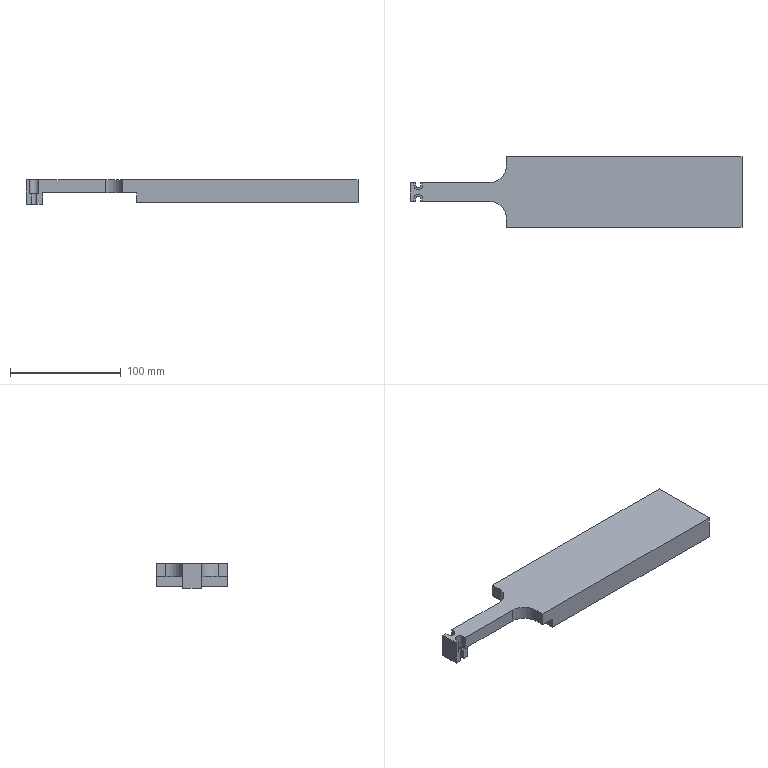Part | SolidWorks | features ICE 4, Fillet 2, Extrusion 1, MirrorPattern 1 | 1 solid | 32 faces | box 300 x 64 x 22.5 mm | volume 298859 mm3 | plane 26 | cylinder 6 | commonest cylinder face diameters 4.5 x2 8 x2 30 x2
STEP:
#1=CARTESIAN_POINT('',(-290.25,-8.5,-1.5));
#2=VERTEX_POINT('',#1);
#3=CARTESIAN_POINT('',(-290.25,-8.5,8.));
#4=VERTEX_POINT('',#3);
#5=CARTESIAN_POINT('',(-290.25,-8.5,-1.501));
#6=DIRECTION('',(0.,0.,1.));
#7=VECTOR('',#6,1000.);
#8=LINE('',#5,#7);
#9=EDGE_CURVE('',#2,#4,#8,.T.);
#10=ORIENTED_EDGE('',*,*,#9,.F.);
#11=CARTESIAN_POINT('',(-285.,-8.5,-1.5));
#12=VERTEX_POINT('',#11);
#13=CARTESIAN_POINT('',(-300.,-8.5,-1.5));
#14=DIRECTION('',(1.,0.,0.));
#15=VECTOR('',#14,1000.);
#16=LINE('',#13,#15);
#17=EDGE_CURVE('',#2,#12,#16,.T.);
#18=ORIENTED_EDGE('',*,*,#17,.T.);
#19=CARTESIAN_POINT('',(-285.,-8.5,9.));
#20=VERTEX_POINT('',#19);
#21=CARTESIAN_POINT('',(-285.,-8.5,9.));
#22=DIRECTION('',(0.,0.,-1.));
#23=VECTOR('',#22,1000.);
#24=LINE('',#21,#23);
#25=EDGE_CURVE('',#20,#12,#24,.T.);
#26=ORIENTED_EDGE('',*,*,#25,.F.);
#27=CARTESIAN_POINT('',(-228.,-8.5,9.));
#28=VERTEX_POINT('',#27);
#29=CARTESIAN_POINT('',(-200.,-8.5,9.));
#30=DIRECTION('',(-1.,0.,0.));
#31=VECTOR('',#30,1000.);
#32=LINE('',#29,#31);
#33=EDGE_CURVE('',#28,#20,#32,.T.);
#34=ORIENTED_EDGE('',*,*,#33,.F.);
#35=CARTESIAN_POINT('',(-228.,-8.5,21.));
#36=VERTEX_POINT('',#35);
#37=CARTESIAN_POINT('',(-228.,-8.5,21.));
#38=DIRECTION('',(0.,0.,1.));
#39=VECTOR('',#38,1000.);
#40=LINE('',#37,#39);
#41=EDGE_CURVE('',#28,#36,#40,.T.);
#42=ORIENTED_EDGE('',*,*,#41,.T.);
#43=CARTESIAN_POINT('',(-288.5,-8.5,21.));
#44=VERTEX_POINT('',#43);
#45=CARTESIAN_POINT('',(-300.,-8.5,21.));
#46=DIRECTION('',(-1.,0.,0.));
#47=VECTOR('',#46,1000.);
#48=LINE('',#45,#47);
#49=EDGE_CURVE('',#36,#44,#48,.T.);
#50=ORIENTED_EDGE('',*,*,#49,.T.);
#51=CARTESIAN_POINT('',(-288.5,-8.5,8.));
#52=VERTEX_POINT('',#51);
#53=CARTESIAN_POINT('',(-288.5,-8.5,8.));
#54=DIRECTION('',(0.,0.,1.));
#55=VECTOR('',#54,1000.);
#56=LINE('',#53,#55);
#57=EDGE_CURVE('',#52,#44,#56,.T.);
#58=ORIENTED_EDGE('',*,*,#57,.F.);
#59=CARTESIAN_POINT('',(-288.5,-8.5,8.));
#60=DIRECTION('',(-1.,0.,0.));
#61=VECTOR('',#60,1000.);
#62=LINE('',#59,#61);
#63=EDGE_CURVE('',#52,#4,#62,.T.);
#64=ORIENTED_EDGE('',*,*,#63,.T.);
#65=EDGE_LOOP('',(#10,#18,#26,#34,#42,#50,#58,#64));
#66=FACE_OUTER_BOUND('',#65,.T.);
#67=CARTESIAN_POINT('',(-300.,-8.5,111.118));
#68=DIRECTION('',(0.,1.,0.));
#69=DIRECTION('',(0.,0.,1.));
#70=AXIS2_PLACEMENT_3D('',#67,#68,#69);
#71=PLANE('',#70);
#72=ADVANCED_FACE('',(#66),#71,.F.);
#73=CARTESIAN_POINT('',(-294.75,-8.5,-1.5));
#74=VERTEX_POINT('',#73);
#75=CARTESIAN_POINT('',(-294.75,-8.5,8.));
#76=VERTEX_POINT('',#75);
#77=CARTESIAN_POINT('',(-294.75,-8.5,-1.501));
#78=DIRECTION('',(0.,0.,1.));
#79=VECTOR('',#78,1000.);
#80=LINE('',#77,#79);
#81=EDGE_CURVE('',#74,#76,#80,.T.);
#82=ORIENTED_EDGE('',*,*,#81,.T.);
#83=CARTESIAN_POINT('',(-296.5,-8.5,8.));
#84=VERTEX_POINT('',#83);
#85=CARTESIAN_POINT('',(-288.5,-8.5,8.));
#86=DIRECTION('',(-1.,0.,0.));
#87=VECTOR('',#86,1000.);
#88=LINE('',#85,#87);
#89=EDGE_CURVE('',#76,#84,#88,.T.);
#90=ORIENTED_EDGE('',*,*,#89,.T.);
#91=CARTESIAN_POINT('',(-296.5,-8.5,21.));
#92=VERTEX_POINT('',#91);
#93=CARTESIAN_POINT('',(-296.5,-8.5,8.));
#94=DIRECTION('',(0.,0.,1.));
#95=VECTOR('',#94,1000.);
#96=LINE('',#93,#95);
#97=EDGE_CURVE('',#84,#92,#96,.T.);
#98=ORIENTED_EDGE('',*,*,#97,.T.);
#99=CARTESIAN_POINT('',(-300.,-8.5,21.));
#100=VERTEX_POINT('',#99);
#101=CARTESIAN_POINT('',(-300.,-8.5,21.));
#102=DIRECTION('',(-1.,0.,0.));
#103=VECTOR('',#102,1000.);
#104=LINE('',#101,#103);
#105=EDGE_CURVE('',#92,#100,#104,.T.);
#106=ORIENTED_EDGE('',*,*,#105,.T.);
#107=CARTESIAN_POINT('',(-300.,-8.5,-1.5));
#108=VERTEX_POINT('',#107);
#109=CARTESIAN_POINT('',(-300.,-8.5,111.118));
#110=DIRECTION('',(0.,0.,-1.));
#111=VECTOR('',#110,1000.);
#112=LINE('',#109,#111);
#113=EDGE_CURVE('',#100,#108,#112,.T.);
#114=ORIENTED_EDGE('',*,*,#113,.T.);
#115=CARTESIAN_POINT('',(-300.,-8.5,-1.5));
#116=DIRECTION('',(1.,0.,0.));
#117=VECTOR('',#116,1000.);
#118=LINE('',#115,#117);
#119=EDGE_CURVE('',#108,#74,#118,.T.);
#120=ORIENTED_EDGE('',*,*,#119,.T.);
#121=EDGE_LOOP('',(#82,#90,#98,#106,#114,#120));
#122=FACE_OUTER_BOUND('',#121,.T.);
#123=CARTESIAN_POINT('',(-300.,-8.5,111.118));
#124=DIRECTION('',(0.,1.,0.));
#125=DIRECTION('',(0.,0.,1.));
#126=AXIS2_PLACEMENT_3D('',#123,#124,#125);
#127=PLANE('',#126);
#128=ADVANCED_FACE('',(#122),#127,.F.);
#129=CARTESIAN_POINT('',(-290.25,-6.1,-1.5));
#130=VERTEX_POINT('',#129);
#131=CARTESIAN_POINT('',(-290.25,-6.1,-1.5));
#132=DIRECTION('',(0.,1.,0.));
#133=VECTOR('',#132,1000.);
#134=LINE('',#131,#133);
#135=EDGE_CURVE('',#2,#130,#134,.T.);
#136=ORIENTED_EDGE('',*,*,#135,.T.);
#137=CARTESIAN_POINT('',(-294.75,-6.1,-1.5));
#138=VERTEX_POINT('',#137);
#139=CARTESIAN_POINT('',(-292.5,-6.1,-1.5));
#140=DIRECTION('',(0.,0.,1.));
#141=DIRECTION('',(1.,0.,0.));
#142=AXIS2_PLACEMENT_3D('',#139,#140,#141);
#143=CIRCLE('',#142,2.25);
#144=EDGE_CURVE('',#130,#138,#143,.T.);
#145=ORIENTED_EDGE('',*,*,#144,.T.);
#146=CARTESIAN_POINT('',(-294.75,-8.5,-1.5));
#147=DIRECTION('',(0.,-1.,0.));
#148=VECTOR('',#147,1000.);
#149=LINE('',#146,#148);
#150=EDGE_CURVE('',#138,#74,#149,.T.);
#151=ORIENTED_EDGE('',*,*,#150,.T.);
#152=ORIENTED_EDGE('',*,*,#119,.F.);
#153=CARTESIAN_POINT('',(-300.,8.5,-1.5));
#154=VERTEX_POINT('',#153);
#155=CARTESIAN_POINT('',(-300.,32.,-1.5));
#156=DIRECTION('',(0.,-1.,0.));
#157=VECTOR('',#156,1000.);
#158=LINE('',#155,#157);
#159=EDGE_CURVE('',#154,#108,#158,.T.);
#160=ORIENTED_EDGE('',*,*,#159,.F.);
#161=CARTESIAN_POINT('',(-294.75,8.5,-1.5));
#162=VERTEX_POINT('',#161);
#163=CARTESIAN_POINT('',(-300.,8.5,-1.5));
#164=DIRECTION('',(-1.,0.,0.));
#165=VECTOR('',#164,1000.);
#166=LINE('',#163,#165);
#167=EDGE_CURVE('',#162,#154,#166,.T.);
#168=ORIENTED_EDGE('',*,*,#167,.F.);
#169=CARTESIAN_POINT('',(-294.75,6.1,-1.5));
#170=VERTEX_POINT('',#169);
#171=CARTESIAN_POINT('',(-294.75,8.5,-1.5));
#172=DIRECTION('',(0.,1.,0.));
#173=VECTOR('',#172,1000.);
#174=LINE('',#171,#173);
#175=EDGE_CURVE('',#170,#162,#174,.T.);
#176=ORIENTED_EDGE('',*,*,#175,.F.);
#177=CARTESIAN_POINT('',(-290.25,6.1,-1.5));
#178=VERTEX_POINT('',#177);
#179=CARTESIAN_POINT('',(-292.5,6.1,-1.5));
#180=DIRECTION('',(0.,0.,-1.));
#181=DIRECTION('',(1.,0.,0.));
#182=AXIS2_PLACEMENT_3D('',#179,#180,#181);
#183=CIRCLE('',#182,2.25);
#184=EDGE_CURVE('',#178,#170,#183,.T.);
#185=ORIENTED_EDGE('',*,*,#184,.F.);
#186=CARTESIAN_POINT('',(-290.25,8.5,-1.5));
#187=VERTEX_POINT('',#186);
#188=CARTESIAN_POINT('',(-290.25,6.1,-1.5));
#189=DIRECTION('',(0.,-1.,0.));
#190=VECTOR('',#189,1000.);
#191=LINE('',#188,#190);
#192=EDGE_CURVE('',#187,#178,#191,.T.);
#193=ORIENTED_EDGE('',*,*,#192,.F.);
#194=CARTESIAN_POINT('',(-285.,8.5,-1.5));
#195=VERTEX_POINT('',#194);
#196=CARTESIAN_POINT('',(-300.,8.5,-1.5));
#197=DIRECTION('',(-1.,0.,0.));
#198=VECTOR('',#197,1000.);
#199=LINE('',#196,#198);
#200=EDGE_CURVE('',#195,#187,#199,.T.);
#201=ORIENTED_EDGE('',*,*,#200,.F.);
#202=CARTESIAN_POINT('',(-285.,32.,-1.5));
#203=DIRECTION('',(0.,-1.,0.));
#204=VECTOR('',#203,1000.);
#205=LINE('',#202,#204);
#206=EDGE_CURVE('',#195,#12,#205,.T.);
#207=ORIENTED_EDGE('',*,*,#206,.T.);
#208=ORIENTED_EDGE('',*,*,#17,.F.);
#209=EDGE_LOOP('',(#136,#145,#151,#152,#160,#168,#176,#185,#193,#201,#207,#208));
#210=FACE_OUTER_BOUND('',#209,.T.);
#211=CARTESIAN_POINT('',(-285.,32.,-1.5));
#212=DIRECTION('',(0.,0.,1.));
#213=DIRECTION('',(1.,0.,0.));
#214=AXIS2_PLACEMENT_3D('',#211,#212,#213);
#215=PLANE('',#214);
#216=ADVANCED_FACE('',(#210),#215,.F.);
#217=CARTESIAN_POINT('',(-294.75,-6.1,8.));
#218=VERTEX_POINT('',#217);
#219=CARTESIAN_POINT('',(-290.25,-6.1,8.));
#220=VERTEX_POINT('',#219);
#221=CARTESIAN_POINT('',(-292.5,-6.1,8.));
#222=DIRECTION('',(0.,0.,-1.));
#223=DIRECTION('',(1.,0.,0.));
#224=AXIS2_PLACEMENT_3D('',#221,#222,#223);
#225=CIRCLE('',#224,2.25);
#226=EDGE_CURVE('',#218,#220,#225,.T.);
#227=ORIENTED_EDGE('',*,*,#226,.T.);
#228=CARTESIAN_POINT('',(-290.25,-6.1,8.));
#229=DIRECTION('',(0.,-1.,0.));
#230=VECTOR('',#229,1000.);
#231=LINE('',#228,#230);
#232=EDGE_CURVE('',#220,#4,#231,.T.);
#233=ORIENTED_EDGE('',*,*,#232,.T.);
#234=ORIENTED_EDGE('',*,*,#63,.F.);
#235=CARTESIAN_POINT('',(-288.5,-6.1,8.));
#236=VERTEX_POINT('',#235);
#237=CARTESIAN_POINT('',(-288.5,-6.1,8.));
#238=DIRECTION('',(0.,-1.,0.));
#239=VECTOR('',#238,1000.);
#240=LINE('',#237,#239);
#241=EDGE_CURVE('',#236,#52,#240,.T.);
#242=ORIENTED_EDGE('',*,*,#241,.F.);
#243=CARTESIAN_POINT('',(-296.5,-6.1,8.));
#244=VERTEX_POINT('',#243);
#245=CARTESIAN_POINT('',(-292.5,-6.1,8.));
#246=DIRECTION('',(0.,0.,-1.));
#247=DIRECTION('',(1.,0.,0.));
#248=AXIS2_PLACEMENT_3D('',#245,#246,#247);
#249=CIRCLE('',#248,4.);
#250=EDGE_CURVE('',#244,#236,#249,.T.);
#251=ORIENTED_EDGE('',*,*,#250,.F.);
#252=CARTESIAN_POINT('',(-296.5,-8.5,8.));
#253=DIRECTION('',(0.,1.,0.));
#254=VECTOR('',#253,1000.);
#255=LINE('',#252,#254);
#256=EDGE_CURVE('',#84,#244,#255,.T.);
#257=ORIENTED_EDGE('',*,*,#256,.F.);
#258=ORIENTED_EDGE('',*,*,#89,.F.);
#259=CARTESIAN_POINT('',(-294.75,-8.5,8.));
#260=DIRECTION('',(0.,1.,0.));
#261=VECTOR('',#260,1000.);
#262=LINE('',#259,#261);
#263=EDGE_CURVE('',#76,#218,#262,.T.);
#264=ORIENTED_EDGE('',*,*,#263,.T.);
#265=EDGE_LOOP('',(#227,#233,#234,#242,#251,#257,#258,#264));
#266=FACE_OUTER_BOUND('',#265,.T.);
#267=CARTESIAN_POINT('',(-292.5,-6.1,8.));
#268=DIRECTION('',(0.,0.,1.));
#269=DIRECTION('',(1.,0.,0.));
#270=AXIS2_PLACEMENT_3D('',#267,#268,#269);
#271=PLANE('',#270);
#272=ADVANCED_FACE('',(#266),#271,.T.);
#273=CARTESIAN_POINT('',(-296.5,-6.1,21.));
#274=VERTEX_POINT('',#273);
#275=CARTESIAN_POINT('',(-296.5,-8.5,21.));
#276=DIRECTION('',(0.,1.,0.));
#277=VECTOR('',#276,1000.);
#278=LINE('',#275,#277);
#279=EDGE_CURVE('',#92,#274,#278,.T.);
#280=ORIENTED_EDGE('',*,*,#279,.T.);
#281=CARTESIAN_POINT('',(-288.5,-6.1,21.));
#282=VERTEX_POINT('',#281);
#283=CARTESIAN_POINT('',(-292.5,-6.1,21.));
#284=DIRECTION('',(0.,0.,-1.));
#285=DIRECTION('',(1.,0.,0.));
#286=AXIS2_PLACEMENT_3D('',#283,#284,#285);
#287=CIRCLE('',#286,4.);
#288=EDGE_CURVE('',#274,#282,#287,.T.);
#289=ORIENTED_EDGE('',*,*,#288,.T.);
#290=CARTESIAN_POINT('',(-288.5,-6.1,21.));
#291=DIRECTION('',(0.,-1.,0.));
#292=VECTOR('',#291,1000.);
#293=LINE('',#290,#292);
#294=EDGE_CURVE('',#282,#44,#293,.T.);
#295=ORIENTED_EDGE('',*,*,#294,.T.);
#296=ORIENTED_EDGE('',*,*,#49,.F.);
#297=CARTESIAN_POINT('',(-213.,-23.5,21.));
#298=VERTEX_POINT('',#297);
#299=CARTESIAN_POINT('',(-228.,-23.5,21.));
#300=DIRECTION('',(0.,0.,-1.));
#301=DIRECTION('',(-1.,0.,0.));
#302=AXIS2_PLACEMENT_3D('',#299,#300,#301);
#303=CIRCLE('',#302,15.);
#304=EDGE_CURVE('',#36,#298,#303,.T.);
#305=ORIENTED_EDGE('',*,*,#304,.T.);
#306=CARTESIAN_POINT('',(-213.,-32.,21.));
#307=VERTEX_POINT('',#306);
#308=CARTESIAN_POINT('',(-213.,-32.,21.));
#309=DIRECTION('',(0.,1.,0.));
#310=VECTOR('',#309,1000.);
#311=LINE('',#308,#310);
#312=EDGE_CURVE('',#307,#298,#311,.T.);
#313=ORIENTED_EDGE('',*,*,#312,.F.);
#314=CARTESIAN_POINT('',(0.,-32.,21.));
#315=VERTEX_POINT('',#314);
#316=CARTESIAN_POINT('',(-300.,-32.,21.));
#317=DIRECTION('',(1.,0.,0.));
#318=VECTOR('',#317,1000.);
#319=LINE('',#316,#318);
#320=EDGE_CURVE('',#307,#315,#319,.T.);
#321=ORIENTED_EDGE('',*,*,#320,.T.);
#322=CARTESIAN_POINT('',(0.,32.,21.));
#323=VERTEX_POINT('',#322);
#324=CARTESIAN_POINT('',(0.,32.,21.));
#325=DIRECTION('',(0.,-1.,0.));
#326=VECTOR('',#325,1000.);
#327=LINE('',#324,#326);
#328=EDGE_CURVE('',#323,#315,#327,.T.);
#329=ORIENTED_EDGE('',*,*,#328,.F.);
#330=CARTESIAN_POINT('',(-213.,32.,21.));
#331=VERTEX_POINT('',#330);
#332=CARTESIAN_POINT('',(-300.,32.,21.));
#333=DIRECTION('',(1.,0.,0.));
#334=VECTOR('',#333,1000.);
#335=LINE('',#332,#334);
#336=EDGE_CURVE('',#331,#323,#335,.T.);
#337=ORIENTED_EDGE('',*,*,#336,.F.);
#338=CARTESIAN_POINT('',(-213.,23.5,21.));
#339=VERTEX_POINT('',#338);
#340=CARTESIAN_POINT('',(-213.,32.,21.));
#341=DIRECTION('',(0.,1.,0.));
#342=VECTOR('',#341,1000.);
#343=LINE('',#340,#342);
#344=EDGE_CURVE('',#339,#331,#343,.T.);
#345=ORIENTED_EDGE('',*,*,#344,.F.);
#346=CARTESIAN_POINT('',(-228.,8.5,21.));
#347=VERTEX_POINT('',#346);
#348=CARTESIAN_POINT('',(-228.,23.5,21.));
#349=DIRECTION('',(0.,0.,-1.));
#350=DIRECTION('',(-1.,0.,0.));
#351=AXIS2_PLACEMENT_3D('',#348,#349,#350);
#352=CIRCLE('',#351,15.);
#353=EDGE_CURVE('',#339,#347,#352,.T.);
#354=ORIENTED_EDGE('',*,*,#353,.T.);
#355=CARTESIAN_POINT('',(-288.5,8.5,21.));
#356=VERTEX_POINT('',#355);
#357=CARTESIAN_POINT('',(-300.,8.5,21.));
#358=DIRECTION('',(1.,0.,0.));
#359=VECTOR('',#358,1000.);
#360=LINE('',#357,#359);
#361=EDGE_CURVE('',#356,#347,#360,.T.);
#362=ORIENTED_EDGE('',*,*,#361,.F.);
#363=CARTESIAN_POINT('',(-288.5,6.1,21.));
#364=VERTEX_POINT('',#363);
#365=CARTESIAN_POINT('',(-288.5,6.1,21.));
#366=DIRECTION('',(0.,1.,0.));
#367=VECTOR('',#366,1000.);
#368=LINE('',#365,#367);
#369=EDGE_CURVE('',#364,#356,#368,.T.);
#370=ORIENTED_EDGE('',*,*,#369,.F.);
#371=CARTESIAN_POINT('',(-296.5,6.1,21.));
#372=VERTEX_POINT('',#371);
#373=CARTESIAN_POINT('',(-292.5,6.1,21.));
#374=DIRECTION('',(0.,0.,1.));
#375=DIRECTION('',(1.,0.,0.));
#376=AXIS2_PLACEMENT_3D('',#373,#374,#375);
#377=CIRCLE('',#376,4.);
#378=EDGE_CURVE('',#372,#364,#377,.T.);
#379=ORIENTED_EDGE('',*,*,#378,.F.);
#380=CARTESIAN_POINT('',(-296.5,8.5,21.));
#381=VERTEX_POINT('',#380);
#382=CARTESIAN_POINT('',(-296.5,8.5,21.));
#383=DIRECTION('',(0.,-1.,0.));
#384=VECTOR('',#383,1000.);
#385=LINE('',#382,#384);
#386=EDGE_CURVE('',#381,#372,#385,.T.);
#387=ORIENTED_EDGE('',*,*,#386,.F.);
#388=CARTESIAN_POINT('',(-300.,8.5,21.));
#389=VERTEX_POINT('',#388);
#390=CARTESIAN_POINT('',(-300.,8.5,21.));
#391=DIRECTION('',(1.,0.,0.));
#392=VECTOR('',#391,1000.);
#393=LINE('',#390,#392);
#394=EDGE_CURVE('',#389,#381,#393,.T.);
#395=ORIENTED_EDGE('',*,*,#394,.F.);
#396=CARTESIAN_POINT('',(-300.,32.,21.));
#397=DIRECTION('',(0.,-1.,0.));
#398=VECTOR('',#397,1000.);
#399=LINE('',#396,#398);
#400=EDGE_CURVE('',#389,#100,#399,.T.);
#401=ORIENTED_EDGE('',*,*,#400,.T.);
#402=ORIENTED_EDGE('',*,*,#105,.F.);
#403=EDGE_LOOP('',(#280,#289,#295,#296,#305,#313,#321,#329,#337,#345,#354,#362,#370,#379,#387,#395,#401,#402));
#404=FACE_OUTER_BOUND('',#403,.T.);
#405=CARTESIAN_POINT('',(-300.,32.,21.));
#406=DIRECTION('',(0.,0.,-1.));
#407=DIRECTION('',(-1.,0.,0.));
#408=AXIS2_PLACEMENT_3D('',#405,#406,#407);
#409=PLANE('',#408);
#410=ADVANCED_FACE('',(#404),#409,.F.);
#411=CARTESIAN_POINT('',(-294.75,8.5,8.));
#412=VERTEX_POINT('',#411);
#413=CARTESIAN_POINT('',(-296.5,8.5,8.));
#414=VERTEX_POINT('',#413);
#415=CARTESIAN_POINT('',(-288.5,8.5,8.));
#416=DIRECTION('',(-1.,0.,0.));
#417=VECTOR('',#416,1000.);
#418=LINE('',#415,#417);
#419=EDGE_CURVE('',#412,#414,#418,.T.);
#420=ORIENTED_EDGE('',*,*,#419,.F.);
#421=CARTESIAN_POINT('',(-294.75,8.5,-1.501));
#422=DIRECTION('',(0.,0.,1.));
#423=VECTOR('',#422,1000.);
#424=LINE('',#421,#423);
#425=EDGE_CURVE('',#162,#412,#424,.T.);
#426=ORIENTED_EDGE('',*,*,#425,.F.);
#427=ORIENTED_EDGE('',*,*,#167,.T.);
#428=CARTESIAN_POINT('',(-300.,8.5,111.118));
#429=DIRECTION('',(0.,0.,-1.));
#430=VECTOR('',#429,1000.);
#431=LINE('',#428,#430);
#432=EDGE_CURVE('',#389,#154,#431,.T.);
#433=ORIENTED_EDGE('',*,*,#432,.F.);
#434=ORIENTED_EDGE('',*,*,#394,.T.);
#435=CARTESIAN_POINT('',(-296.5,8.5,8.));
#436=DIRECTION('',(0.,0.,1.));
#437=VECTOR('',#436,1000.);
#438=LINE('',#435,#437);
#439=EDGE_CURVE('',#414,#381,#438,.T.);
#440=ORIENTED_EDGE('',*,*,#439,.F.);
#441=EDGE_LOOP('',(#420,#426,#427,#433,#434,#440));
#442=FACE_OUTER_BOUND('',#441,.T.);
#443=CARTESIAN_POINT('',(-300.,8.5,111.118));
#444=DIRECTION('',(0.,-1.,0.));
#445=DIRECTION('',(0.,0.,-1.));
#446=AXIS2_PLACEMENT_3D('',#443,#444,#445);
#447=PLANE('',#446);
#448=ADVANCED_FACE('',(#442),#447,.F.);
#449=CARTESIAN_POINT('',(0.,-32.,0.));
#450=VERTEX_POINT('',#449);
#451=CARTESIAN_POINT('',(0.,-32.,21.));
#452=DIRECTION('',(0.,0.,-1.));
#453=VECTOR('',#452,1000.);
#454=LINE('',#451,#453);
#455=EDGE_CURVE('',#315,#450,#454,.T.);
#456=ORIENTED_EDGE('',*,*,#455,.T.);
#457=CARTESIAN_POINT('',(0.,32.,0.));
#458=VERTEX_POINT('',#457);
#459=CARTESIAN_POINT('',(0.,32.,0.));
#460=DIRECTION('',(0.,-1.,0.));
#461=VECTOR('',#460,1000.);
#462=LINE('',#459,#461);
#463=EDGE_CURVE('',#458,#450,#462,.T.);
#464=ORIENTED_EDGE('',*,*,#463,.F.);
#465=CARTESIAN_POINT('',(0.,32.,21.));
#466=DIRECTION('',(0.,0.,-1.));
#467=VECTOR('',#466,1000.);
#468=LINE('',#465,#467);
#469=EDGE_CURVE('',#323,#458,#468,.T.);
#470=ORIENTED_EDGE('',*,*,#469,.F.);
#471=ORIENTED_EDGE('',*,*,#328,.T.);
#472=EDGE_LOOP('',(#456,#464,#470,#471));
#473=FACE_OUTER_BOUND('',#472,.T.);
#474=CARTESIAN_POINT('',(0.,32.,21.));
#475=DIRECTION('',(-1.,0.,0.));
#476=DIRECTION('',(0.,0.,1.));
#477=AXIS2_PLACEMENT_3D('',#474,#475,#476);
#478=PLANE('',#477);
#479=ADVANCED_FACE('',(#473),#478,.F.);
#480=CARTESIAN_POINT('',(-200.,-32.,0.));
#481=VERTEX_POINT('',#480);
#482=CARTESIAN_POINT('',(0.,-32.,0.));
#483=DIRECTION('',(-1.,0.,0.));
#484=VECTOR('',#483,1000.);
#485=LINE('',#482,#484);
#486=EDGE_CURVE('',#450,#481,#485,.T.);
#487=ORIENTED_EDGE('',*,*,#486,.T.);
#488=CARTESIAN_POINT('',(-200.,32.,0.));
#489=VERTEX_POINT('',#488);
#490=CARTESIAN_POINT('',(-200.,32.,0.));
#491=DIRECTION('',(0.,-1.,0.));
#492=VECTOR('',#491,1000.);
#493=LINE('',#490,#492);
#494=EDGE_CURVE('',#489,#481,#493,.T.);
#495=ORIENTED_EDGE('',*,*,#494,.F.);
#496=CARTESIAN_POINT('',(0.,32.,0.));
#497=DIRECTION('',(-1.,0.,0.));
#498=VECTOR('',#497,1000.);
#499=LINE('',#496,#498);
#500=EDGE_CURVE('',#458,#489,#499,.T.);
#501=ORIENTED_EDGE('',*,*,#500,.F.);
#502=ORIENTED_EDGE('',*,*,#463,.T.);
#503=EDGE_LOOP('',(#487,#495,#501,#502));
#504=FACE_OUTER_BOUND('',#503,.T.);
#505=CARTESIAN_POINT('',(0.,32.,0.));
#506=DIRECTION('',(0.,0.,1.));
#507=DIRECTION('',(1.,0.,0.));
#508=AXIS2_PLACEMENT_3D('',#505,#506,#507);
#509=PLANE('',#508);
#510=ADVANCED_FACE('',(#504),#509,.F.);
#511=CARTESIAN_POINT('',(-200.,-32.,9.));
#512=VERTEX_POINT('',#511);
#513=CARTESIAN_POINT('',(-200.,-32.,0.));
#514=DIRECTION('',(0.,0.,1.));
#515=VECTOR('',#514,1000.);
#516=LINE('',#513,#515);
#517=EDGE_CURVE('',#481,#512,#516,.T.);
#518=ORIENTED_EDGE('',*,*,#517,.T.);
#519=CARTESIAN_POINT('',(-200.,32.,9.));
#520=VERTEX_POINT('',#519);
#521=CARTESIAN_POINT('',(-200.,32.,9.));
#522=DIRECTION('',(0.,-1.,0.));
#523=VECTOR('',#522,1000.);
#524=LINE('',#521,#523);
#525=EDGE_CURVE('',#520,#512,#524,.T.);
#526=ORIENTED_EDGE('',*,*,#525,.F.);
#527=CARTESIAN_POINT('',(-200.,32.,0.));
#528=DIRECTION('',(0.,0.,1.));
#529=VECTOR('',#528,1000.);
#530=LINE('',#527,#529);
#531=EDGE_CURVE('',#489,#520,#530,.T.);
#532=ORIENTED_EDGE('',*,*,#531,.F.);
#533=ORIENTED_EDGE('',*,*,#494,.T.);
#534=EDGE_LOOP('',(#518,#526,#532,#533));
#535=FACE_OUTER_BOUND('',#534,.T.);
#536=CARTESIAN_POINT('',(-200.,32.,0.));
#537=DIRECTION('',(1.,0.,0.));
#538=DIRECTION('',(0.,0.,-1.));
#539=AXIS2_PLACEMENT_3D('',#536,#537,#538);
#540=PLANE('',#539);
#541=ADVANCED_FACE('',(#535),#540,.F.);
#542=CARTESIAN_POINT('',(-213.,-32.,9.));
#543=VERTEX_POINT('',#542);
#544=CARTESIAN_POINT('',(-200.,-32.,9.));
#545=DIRECTION('',(-1.,0.,0.));
#546=VECTOR('',#545,1000.);
#547=LINE('',#544,#546);
#548=EDGE_CURVE('',#512,#543,#547,.T.);
#549=ORIENTED_EDGE('',*,*,#548,.T.);
#550=CARTESIAN_POINT('',(-213.,-23.5,9.));
#551=VERTEX_POINT('',#550);
#552=CARTESIAN_POINT('',(-213.,32.,9.));
#553=DIRECTION('',(0.,1.,0.));
#554=VECTOR('',#553,1000.);
#555=LINE('',#552,#554);
#556=EDGE_CURVE('',#543,#551,#555,.T.);
#557=ORIENTED_EDGE('',*,*,#556,.T.);
#558=CARTESIAN_POINT('',(-228.,-23.5,9.));
#559=DIRECTION('',(0.,0.,1.));
#560=DIRECTION('',(1.,0.,0.));
#561=AXIS2_PLACEMENT_3D('',#558,#559,#560);
#562=CIRCLE('',#561,15.);
#563=EDGE_CURVE('',#551,#28,#562,.T.);
#564=ORIENTED_EDGE('',*,*,#563,.T.);
#565=ORIENTED_EDGE('',*,*,#33,.T.);
#566=CARTESIAN_POINT('',(-285.,8.5,9.));
#567=VERTEX_POINT('',#566);
#568=CARTESIAN_POINT('',(-285.,32.,9.));
#569=DIRECTION('',(0.,-1.,0.));
#570=VECTOR('',#569,1000.);
#571=LINE('',#568,#570);
#572=EDGE_CURVE('',#567,#20,#571,.T.);
#573=ORIENTED_EDGE('',*,*,#572,.F.);
#574=CARTESIAN_POINT('',(-228.,8.5,9.));
#575=VERTEX_POINT('',#574);
#576=CARTESIAN_POINT('',(-200.,8.5,9.));
#577=DIRECTION('',(1.,0.,0.));
#578=VECTOR('',#577,1000.);
#579=LINE('',#576,#578);
#580=EDGE_CURVE('',#567,#575,#579,.T.);
#581=ORIENTED_EDGE('',*,*,#580,.T.);
#582=CARTESIAN_POINT('',(-213.,23.5,9.));
#583=VERTEX_POINT('',#582);
#584=CARTESIAN_POINT('',(-228.,23.5,9.));
#585=DIRECTION('',(0.,0.,1.));
#586=DIRECTION('',(1.,0.,0.));
#587=AXIS2_PLACEMENT_3D('',#584,#585,#586);
#588=CIRCLE('',#587,15.);
#589=EDGE_CURVE('',#575,#583,#588,.T.);
#590=ORIENTED_EDGE('',*,*,#589,.T.);
#591=CARTESIAN_POINT('',(-213.,32.,9.));
#592=VERTEX_POINT('',#591);
#593=CARTESIAN_POINT('',(-213.,32.,9.));
#594=DIRECTION('',(0.,1.,0.));
#595=VECTOR('',#594,1000.);
#596=LINE('',#593,#595);
#597=EDGE_CURVE('',#583,#592,#596,.T.);
#598=ORIENTED_EDGE('',*,*,#597,.T.);
#599=CARTESIAN_POINT('',(-200.,32.,9.));
#600=DIRECTION('',(-1.,0.,0.));
#601=VECTOR('',#600,1000.);
#602=LINE('',#599,#601);
#603=EDGE_CURVE('',#520,#592,#602,.T.);
#604=ORIENTED_EDGE('',*,*,#603,.F.);
#605=ORIENTED_EDGE('',*,*,#525,.T.);
#606=EDGE_LOOP('',(#549,#557,#564,#565,#573,#581,#590,#598,#604,#605));
#607=FACE_OUTER_BOUND('',#606,.T.);
#608=CARTESIAN_POINT('',(-200.,32.,9.));
#609=DIRECTION('',(0.,0.,1.));
#610=DIRECTION('',(1.,0.,0.));
#611=AXIS2_PLACEMENT_3D('',#608,#609,#610);
#612=PLANE('',#611);
#613=ADVANCED_FACE('',(#607),#612,.F.);
#614=ORIENTED_EDGE('',*,*,#572,.T.);
#615=ORIENTED_EDGE('',*,*,#25,.T.);
#616=ORIENTED_EDGE('',*,*,#206,.F.);
#617=CARTESIAN_POINT('',(-285.,8.5,9.));
#618=DIRECTION('',(0.,0.,1.));
#619=VECTOR('',#618,1000.);
#620=LINE('',#617,#619);
#621=EDGE_CURVE('',#195,#567,#620,.T.);
#622=ORIENTED_EDGE('',*,*,#621,.T.);
#623=EDGE_LOOP('',(#614,#615,#616,#622));
#624=FACE_OUTER_BOUND('',#623,.T.);
#625=CARTESIAN_POINT('',(-285.,32.,9.));
#626=DIRECTION('',(-1.,0.,0.));
#627=DIRECTION('',(0.,0.,1.));
#628=AXIS2_PLACEMENT_3D('',#625,#626,#627);
#629=PLANE('',#628);
#630=ADVANCED_FACE('',(#624),#629,.F.);
#631=ORIENTED_EDGE('',*,*,#159,.T.);
#632=ORIENTED_EDGE('',*,*,#113,.F.);
#633=ORIENTED_EDGE('',*,*,#400,.F.);
#634=ORIENTED_EDGE('',*,*,#432,.T.);
#635=EDGE_LOOP('',(#631,#632,#633,#634));
#636=FACE_OUTER_BOUND('',#635,.T.);
#637=CARTESIAN_POINT('',(-300.,32.,-1.5));
#638=DIRECTION('',(1.,0.,0.));
#639=DIRECTION('',(0.,0.,-1.));
#640=AXIS2_PLACEMENT_3D('',#637,#638,#639);
#641=PLANE('',#640);
#642=ADVANCED_FACE('',(#636),#641,.F.);
#643=CARTESIAN_POINT('',(-213.,32.,111.118));
#644=DIRECTION('',(0.,0.,-1.));
#645=VECTOR('',#644,1000.);
#646=LINE('',#643,#645);
#647=EDGE_CURVE('',#331,#592,#646,.T.);
#648=ORIENTED_EDGE('',*,*,#647,.F.);
#649=ORIENTED_EDGE('',*,*,#336,.T.);
#650=ORIENTED_EDGE('',*,*,#469,.T.);
#651=ORIENTED_EDGE('',*,*,#500,.T.);
#652=ORIENTED_EDGE('',*,*,#531,.T.);
#653=ORIENTED_EDGE('',*,*,#603,.T.);
#654=EDGE_LOOP('',(#648,#649,#650,#651,#652,#653));
#655=FACE_OUTER_BOUND('',#654,.T.);
#656=CARTESIAN_POINT('',(0.,32.,0.));
#657=DIRECTION('',(0.,1.,0.));
#658=DIRECTION('',(0.,0.,1.));
#659=AXIS2_PLACEMENT_3D('',#656,#657,#658);
#660=PLANE('',#659);
#661=ADVANCED_FACE('',(#655),#660,.T.);
#662=ORIENTED_EDGE('',*,*,#320,.F.);
#663=CARTESIAN_POINT('',(-213.,-32.,111.118));
#664=DIRECTION('',(0.,0.,-1.));
#665=VECTOR('',#664,1000.);
#666=LINE('',#663,#665);
#667=EDGE_CURVE('',#307,#543,#666,.T.);
#668=ORIENTED_EDGE('',*,*,#667,.T.);
#669=ORIENTED_EDGE('',*,*,#548,.F.);
#670=ORIENTED_EDGE('',*,*,#517,.F.);
#671=ORIENTED_EDGE('',*,*,#486,.F.);
#672=ORIENTED_EDGE('',*,*,#455,.F.);
#673=EDGE_LOOP('',(#662,#668,#669,#670,#671,#672));
#674=FACE_OUTER_BOUND('',#673,.T.);
#675=CARTESIAN_POINT('',(0.,-32.,0.));
#676=DIRECTION('',(0.,1.,0.));
#677=DIRECTION('',(0.,0.,1.));
#678=AXIS2_PLACEMENT_3D('',#675,#676,#677);
#679=PLANE('',#678);
#680=ADVANCED_FACE('',(#674),#679,.F.);
#681=ORIENTED_EDGE('',*,*,#312,.T.);
#682=CARTESIAN_POINT('',(-213.,-23.5,9.));
#683=DIRECTION('',(0.,0.,-1.));
#684=VECTOR('',#683,1000.);
#685=LINE('',#682,#684);
#686=EDGE_CURVE('',#298,#551,#685,.T.);
#687=ORIENTED_EDGE('',*,*,#686,.T.);
#688=ORIENTED_EDGE('',*,*,#556,.F.);
#689=ORIENTED_EDGE('',*,*,#667,.F.);
#690=EDGE_LOOP('',(#681,#687,#688,#689));
#691=FACE_OUTER_BOUND('',#690,.T.);
#692=CARTESIAN_POINT('',(-213.,-32.,111.118));
#693=DIRECTION('',(1.,0.,0.));
#694=DIRECTION('',(0.,0.,-1.));
#695=AXIS2_PLACEMENT_3D('',#692,#693,#694);
#696=PLANE('',#695);
#697=ADVANCED_FACE('',(#691),#696,.F.);
#698=ORIENTED_EDGE('',*,*,#200,.T.);
#699=CARTESIAN_POINT('',(-290.25,8.5,8.));
#700=VERTEX_POINT('',#699);
#701=CARTESIAN_POINT('',(-290.25,8.5,-1.501));
#702=DIRECTION('',(0.,0.,1.));
#703=VECTOR('',#702,1000.);
#704=LINE('',#701,#703);
#705=EDGE_CURVE('',#187,#700,#704,.T.);
#706=ORIENTED_EDGE('',*,*,#705,.T.);
#707=CARTESIAN_POINT('',(-288.5,8.5,8.));
#708=VERTEX_POINT('',#707);
#709=CARTESIAN_POINT('',(-288.5,8.5,8.));
#710=DIRECTION('',(-1.,0.,0.));
#711=VECTOR('',#710,1000.);
#712=LINE('',#709,#711);
#713=EDGE_CURVE('',#708,#700,#712,.T.);
#714=ORIENTED_EDGE('',*,*,#713,.F.);
#715=CARTESIAN_POINT('',(-288.5,8.5,8.));
#716=DIRECTION('',(0.,0.,1.));
#717=VECTOR('',#716,1000.);
#718=LINE('',#715,#717);
#719=EDGE_CURVE('',#708,#356,#718,.T.);
#720=ORIENTED_EDGE('',*,*,#719,.T.);
#721=ORIENTED_EDGE('',*,*,#361,.T.);
#722=CARTESIAN_POINT('',(-228.,8.5,9.));
#723=DIRECTION('',(0.,0.,-1.));
#724=VECTOR('',#723,1000.);
#725=LINE('',#722,#724);
#726=EDGE_CURVE('',#347,#575,#725,.T.);
#727=ORIENTED_EDGE('',*,*,#726,.T.);
#728=ORIENTED_EDGE('',*,*,#580,.F.);
#729=ORIENTED_EDGE('',*,*,#621,.F.);
#730=EDGE_LOOP('',(#698,#706,#714,#720,#721,#727,#728,#729));
#731=FACE_OUTER_BOUND('',#730,.T.);
#732=CARTESIAN_POINT('',(-300.,8.5,111.118));
#733=DIRECTION('',(0.,-1.,0.));
#734=DIRECTION('',(0.,0.,-1.));
#735=AXIS2_PLACEMENT_3D('',#732,#733,#734);
#736=PLANE('',#735);
#737=ADVANCED_FACE('',(#731),#736,.F.);
#738=ORIENTED_EDGE('',*,*,#597,.F.);
#739=CARTESIAN_POINT('',(-213.,23.5,21.));
#740=DIRECTION('',(0.,0.,1.));
#741=VECTOR('',#740,1000.);
#742=LINE('',#739,#741);
#743=EDGE_CURVE('',#583,#339,#742,.T.);
#744=ORIENTED_EDGE('',*,*,#743,.T.);
#745=ORIENTED_EDGE('',*,*,#344,.T.);
#746=ORIENTED_EDGE('',*,*,#647,.T.);
#747=EDGE_LOOP('',(#738,#744,#745,#746));
#748=FACE_OUTER_BOUND('',#747,.T.);
#749=CARTESIAN_POINT('',(-213.,32.,111.118));
#750=DIRECTION('',(1.,0.,0.));
#751=DIRECTION('',(0.,1.,0.));
#752=AXIS2_PLACEMENT_3D('',#749,#750,#751);
#753=PLANE('',#752);
#754=ADVANCED_FACE('',(#748),#753,.F.);
#755=ORIENTED_EDGE('',*,*,#353,.F.);
#756=ORIENTED_EDGE('',*,*,#743,.F.);
#757=ORIENTED_EDGE('',*,*,#589,.F.);
#758=ORIENTED_EDGE('',*,*,#726,.F.);
#759=EDGE_LOOP('',(#755,#756,#757,#758));
#760=FACE_OUTER_BOUND('',#759,.T.);
#761=CARTESIAN_POINT('',(-228.,23.5,111.118));
#762=DIRECTION('',(0.,0.,1.));
#763=DIRECTION('',(1.,0.,0.));
#764=AXIS2_PLACEMENT_3D('',#761,#762,#763);
#765=CYLINDRICAL_SURFACE('',#764,15.);
#766=ADVANCED_FACE('',(#760),#765,.F.);
#767=ORIENTED_EDGE('',*,*,#304,.F.);
#768=ORIENTED_EDGE('',*,*,#41,.F.);
#769=ORIENTED_EDGE('',*,*,#563,.F.);
#770=ORIENTED_EDGE('',*,*,#686,.F.);
#771=EDGE_LOOP('',(#767,#768,#769,#770));
#772=FACE_OUTER_BOUND('',#771,.T.);
#773=CARTESIAN_POINT('',(-228.,-23.5,111.118));
#774=DIRECTION('',(0.,0.,1.));
#775=DIRECTION('',(1.,0.,0.));
#776=AXIS2_PLACEMENT_3D('',#773,#774,#775);
#777=CYLINDRICAL_SURFACE('',#776,15.);
#778=ADVANCED_FACE('',(#772),#777,.F.);
#779=ORIENTED_EDGE('',*,*,#369,.T.);
#780=ORIENTED_EDGE('',*,*,#719,.F.);
#781=CARTESIAN_POINT('',(-288.5,6.1,8.));
#782=VERTEX_POINT('',#781);
#783=CARTESIAN_POINT('',(-288.5,6.1,8.));
#784=DIRECTION('',(0.,1.,0.));
#785=VECTOR('',#784,1000.);
#786=LINE('',#783,#785);
#787=EDGE_CURVE('',#782,#708,#786,.T.);
#788=ORIENTED_EDGE('',*,*,#787,.F.);
#789=CARTESIAN_POINT('',(-288.5,6.1,8.));
#790=DIRECTION('',(0.,0.,1.));
#791=VECTOR('',#790,1000.);
#792=LINE('',#789,#791);
#793=EDGE_CURVE('',#782,#364,#792,.T.);
#794=ORIENTED_EDGE('',*,*,#793,.T.);
#795=EDGE_LOOP('',(#779,#780,#788,#794));
#796=FACE_OUTER_BOUND('',#795,.T.);
#797=CARTESIAN_POINT('',(-288.5,6.1,8.));
#798=DIRECTION('',(1.,0.,0.));
#799=DIRECTION('',(0.,0.,-1.));
#800=AXIS2_PLACEMENT_3D('',#797,#798,#799);
#801=PLANE('',#800);
#802=ADVANCED_FACE('',(#796),#801,.F.);
#803=ORIENTED_EDGE('',*,*,#378,.T.);
#804=ORIENTED_EDGE('',*,*,#793,.F.);
#805=CARTESIAN_POINT('',(-296.5,6.1,8.));
#806=VERTEX_POINT('',#805);
#807=CARTESIAN_POINT('',(-292.5,6.1,8.));
#808=DIRECTION('',(0.,0.,1.));
#809=DIRECTION('',(1.,0.,0.));
#810=AXIS2_PLACEMENT_3D('',#807,#808,#809);
#811=CIRCLE('',#810,4.);
#812=EDGE_CURVE('',#806,#782,#811,.T.);
#813=ORIENTED_EDGE('',*,*,#812,.F.);
#814=CARTESIAN_POINT('',(-296.5,6.1,8.));
#815=DIRECTION('',(0.,0.,1.));
#816=VECTOR('',#815,1000.);
#817=LINE('',#814,#816);
#818=EDGE_CURVE('',#806,#372,#817,.T.);
#819=ORIENTED_EDGE('',*,*,#818,.T.);
#820=EDGE_LOOP('',(#803,#804,#813,#819));
#821=FACE_OUTER_BOUND('',#820,.T.);
#822=CARTESIAN_POINT('',(-292.5,6.1,8.));
#823=DIRECTION('',(0.,0.,1.));
#824=DIRECTION('',(1.,0.,0.));
#825=AXIS2_PLACEMENT_3D('',#822,#823,#824);
#826=CYLINDRICAL_SURFACE('',#825,4.);
#827=ADVANCED_FACE('',(#821),#826,.F.);
#828=ORIENTED_EDGE('',*,*,#386,.T.);
#829=ORIENTED_EDGE('',*,*,#818,.F.);
#830=CARTESIAN_POINT('',(-296.5,8.5,8.));
#831=DIRECTION('',(0.,-1.,0.));
#832=VECTOR('',#831,1000.);
#833=LINE('',#830,#832);
#834=EDGE_CURVE('',#414,#806,#833,.T.);
#835=ORIENTED_EDGE('',*,*,#834,.F.);
#836=ORIENTED_EDGE('',*,*,#439,.T.);
#837=EDGE_LOOP('',(#828,#829,#835,#836));
#838=FACE_OUTER_BOUND('',#837,.T.);
#839=CARTESIAN_POINT('',(-296.5,8.5,8.));
#840=DIRECTION('',(-1.,0.,0.));
#841=DIRECTION('',(0.,0.,1.));
#842=AXIS2_PLACEMENT_3D('',#839,#840,#841);
#843=PLANE('',#842);
#844=ADVANCED_FACE('',(#838),#843,.F.);
#845=CARTESIAN_POINT('',(-294.75,6.1,8.));
#846=VERTEX_POINT('',#845);
#847=CARTESIAN_POINT('',(-294.75,8.5,8.));
#848=DIRECTION('',(0.,-1.,0.));
#849=VECTOR('',#848,1000.);
#850=LINE('',#847,#849);
#851=EDGE_CURVE('',#412,#846,#850,.T.);
#852=ORIENTED_EDGE('',*,*,#851,.F.);
#853=ORIENTED_EDGE('',*,*,#419,.T.);
#854=ORIENTED_EDGE('',*,*,#834,.T.);
#855=ORIENTED_EDGE('',*,*,#812,.T.);
#856=ORIENTED_EDGE('',*,*,#787,.T.);
#857=ORIENTED_EDGE('',*,*,#713,.T.);
#858=CARTESIAN_POINT('',(-290.25,6.1,8.));
#859=VERTEX_POINT('',#858);
#860=CARTESIAN_POINT('',(-290.25,6.1,8.));
#861=DIRECTION('',(0.,1.,0.));
#862=VECTOR('',#861,1000.);
#863=LINE('',#860,#862);
#864=EDGE_CURVE('',#859,#700,#863,.T.);
#865=ORIENTED_EDGE('',*,*,#864,.F.);
#866=CARTESIAN_POINT('',(-292.5,6.1,8.));
#867=DIRECTION('',(0.,0.,1.));
#868=DIRECTION('',(1.,0.,0.));
#869=AXIS2_PLACEMENT_3D('',#866,#867,#868);
#870=CIRCLE('',#869,2.25);
#871=EDGE_CURVE('',#846,#859,#870,.T.);
#872=ORIENTED_EDGE('',*,*,#871,.F.);
#873=EDGE_LOOP('',(#852,#853,#854,#855,#856,#857,#865,#872));
#874=FACE_OUTER_BOUND('',#873,.T.);
#875=CARTESIAN_POINT('',(-292.5,6.1,8.));
#876=DIRECTION('',(0.,0.,1.));
#877=DIRECTION('',(1.,0.,0.));
#878=AXIS2_PLACEMENT_3D('',#875,#876,#877);
#879=PLANE('',#878);
#880=ADVANCED_FACE('',(#874),#879,.T.);
#881=ORIENTED_EDGE('',*,*,#184,.T.);
#882=CARTESIAN_POINT('',(-294.75,6.1,-1.501));
#883=DIRECTION('',(0.,0.,1.));
#884=VECTOR('',#883,1000.);
#885=LINE('',#882,#884);
#886=EDGE_CURVE('',#170,#846,#885,.T.);
#887=ORIENTED_EDGE('',*,*,#886,.T.);
#888=ORIENTED_EDGE('',*,*,#871,.T.);
#889=CARTESIAN_POINT('',(-290.25,6.1,-1.501));
#890=DIRECTION('',(0.,0.,1.));
#891=VECTOR('',#890,1000.);
#892=LINE('',#889,#891);
#893=EDGE_CURVE('',#178,#859,#892,.T.);
#894=ORIENTED_EDGE('',*,*,#893,.F.);
#895=EDGE_LOOP('',(#881,#887,#888,#894));
#896=FACE_OUTER_BOUND('',#895,.T.);
#897=CARTESIAN_POINT('',(-292.5,6.1,-1.501));
#898=DIRECTION('',(0.,0.,1.));
#899=DIRECTION('',(1.,0.,0.));
#900=AXIS2_PLACEMENT_3D('',#897,#898,#899);
#901=CYLINDRICAL_SURFACE('',#900,2.25);
#902=ADVANCED_FACE('',(#896),#901,.F.);
#903=ORIENTED_EDGE('',*,*,#175,.T.);
#904=ORIENTED_EDGE('',*,*,#425,.T.);
#905=ORIENTED_EDGE('',*,*,#851,.T.);
#906=ORIENTED_EDGE('',*,*,#886,.F.);
#907=EDGE_LOOP('',(#903,#904,#905,#906));
#908=FACE_OUTER_BOUND('',#907,.T.);
#909=CARTESIAN_POINT('',(-294.75,8.5,-1.501));
#910=DIRECTION('',(-1.,0.,0.));
#911=DIRECTION('',(0.,0.,1.));
#912=AXIS2_PLACEMENT_3D('',#909,#910,#911);
#913=PLANE('',#912);
#914=ADVANCED_FACE('',(#908),#913,.F.);
#915=ORIENTED_EDGE('',*,*,#192,.T.);
#916=ORIENTED_EDGE('',*,*,#893,.T.);
#917=ORIENTED_EDGE('',*,*,#864,.T.);
#918=ORIENTED_EDGE('',*,*,#705,.F.);
#919=EDGE_LOOP('',(#915,#916,#917,#918));
#920=FACE_OUTER_BOUND('',#919,.T.);
#921=CARTESIAN_POINT('',(-290.25,6.1,-1.501));
#922=DIRECTION('',(1.,0.,0.));
#923=DIRECTION('',(0.,1.,0.));
#924=AXIS2_PLACEMENT_3D('',#921,#922,#923);
#925=PLANE('',#924);
#926=ADVANCED_FACE('',(#920),#925,.F.);
#927=ORIENTED_EDGE('',*,*,#279,.F.);
#928=ORIENTED_EDGE('',*,*,#97,.F.);
#929=ORIENTED_EDGE('',*,*,#256,.T.);
#930=CARTESIAN_POINT('',(-296.5,-6.1,8.));
#931=DIRECTION('',(0.,0.,1.));
#932=VECTOR('',#931,1000.);
#933=LINE('',#930,#932);
#934=EDGE_CURVE('',#244,#274,#933,.T.);
#935=ORIENTED_EDGE('',*,*,#934,.T.);
#936=EDGE_LOOP('',(#927,#928,#929,#935));
#937=FACE_OUTER_BOUND('',#936,.T.);
#938=CARTESIAN_POINT('',(-296.5,-8.5,8.));
#939=DIRECTION('',(1.,0.,0.));
#940=DIRECTION('',(0.,0.,-1.));
#941=AXIS2_PLACEMENT_3D('',#938,#939,#940);
#942=PLANE('',#941);
#943=ADVANCED_FACE('',(#937),#942,.T.);
#944=ORIENTED_EDGE('',*,*,#288,.F.);
#945=ORIENTED_EDGE('',*,*,#934,.F.);
#946=ORIENTED_EDGE('',*,*,#250,.T.);
#947=CARTESIAN_POINT('',(-288.5,-6.1,8.));
#948=DIRECTION('',(0.,0.,1.));
#949=VECTOR('',#948,1000.);
#950=LINE('',#947,#949);
#951=EDGE_CURVE('',#236,#282,#950,.T.);
#952=ORIENTED_EDGE('',*,*,#951,.T.);
#953=EDGE_LOOP('',(#944,#945,#946,#952));
#954=FACE_OUTER_BOUND('',#953,.T.);
#955=CARTESIAN_POINT('',(-292.5,-6.1,8.));
#956=DIRECTION('',(0.,0.,1.));
#957=DIRECTION('',(1.,0.,0.));
#958=AXIS2_PLACEMENT_3D('',#955,#956,#957);
#959=CYLINDRICAL_SURFACE('',#958,4.);
#960=ADVANCED_FACE('',(#954),#959,.F.);
#961=ORIENTED_EDGE('',*,*,#294,.F.);
#962=ORIENTED_EDGE('',*,*,#951,.F.);
#963=ORIENTED_EDGE('',*,*,#241,.T.);
#964=ORIENTED_EDGE('',*,*,#57,.T.);
#965=EDGE_LOOP('',(#961,#962,#963,#964));
#966=FACE_OUTER_BOUND('',#965,.T.);
#967=CARTESIAN_POINT('',(-288.5,-6.1,8.));
#968=DIRECTION('',(-1.,0.,0.));
#969=DIRECTION('',(0.,0.,1.));
#970=AXIS2_PLACEMENT_3D('',#967,#968,#969);
#971=PLANE('',#970);
#972=ADVANCED_FACE('',(#966),#971,.T.);
#973=CARTESIAN_POINT('',(-290.25,-6.1,-1.501));
#974=DIRECTION('',(0.,0.,1.));
#975=VECTOR('',#974,1000.);
#976=LINE('',#973,#975);
#977=EDGE_CURVE('',#130,#220,#976,.T.);
#978=ORIENTED_EDGE('',*,*,#977,.T.);
#979=ORIENTED_EDGE('',*,*,#226,.F.);
#980=CARTESIAN_POINT('',(-294.75,-6.1,-1.501));
#981=DIRECTION('',(0.,0.,1.));
#982=VECTOR('',#981,1000.);
#983=LINE('',#980,#982);
#984=EDGE_CURVE('',#138,#218,#983,.T.);
#985=ORIENTED_EDGE('',*,*,#984,.F.);
#986=ORIENTED_EDGE('',*,*,#144,.F.);
#987=EDGE_LOOP('',(#978,#979,#985,#986));
#988=FACE_OUTER_BOUND('',#987,.T.);
#989=CARTESIAN_POINT('',(-292.5,-6.1,-1.501));
#990=DIRECTION('',(0.,0.,1.));
#991=DIRECTION('',(1.,0.,0.));
#992=AXIS2_PLACEMENT_3D('',#989,#990,#991);
#993=CYLINDRICAL_SURFACE('',#992,2.25);
#994=ADVANCED_FACE('',(#988),#993,.F.);
#995=ORIENTED_EDGE('',*,*,#9,.T.);
#996=ORIENTED_EDGE('',*,*,#232,.F.);
#997=ORIENTED_EDGE('',*,*,#977,.F.);
#998=ORIENTED_EDGE('',*,*,#135,.F.);
#999=EDGE_LOOP('',(#995,#996,#997,#998));
#1000=FACE_OUTER_BOUND('',#999,.T.);
#1001=CARTESIAN_POINT('',(-290.25,-6.1,-1.501));
#1002=DIRECTION('',(-1.,0.,0.));
#1003=DIRECTION('',(0.,-1.,0.));
#1004=AXIS2_PLACEMENT_3D('',#1001,#1002,#1003);
#1005=PLANE('',#1004);
#1006=ADVANCED_FACE('',(#1000),#1005,.T.);
#1007=ORIENTED_EDGE('',*,*,#984,.T.);
#1008=ORIENTED_EDGE('',*,*,#263,.F.);
#1009=ORIENTED_EDGE('',*,*,#81,.F.);
#1010=ORIENTED_EDGE('',*,*,#150,.F.);
#1011=EDGE_LOOP('',(#1007,#1008,#1009,#1010));
#1012=FACE_OUTER_BOUND('',#1011,.T.);
#1013=CARTESIAN_POINT('',(-294.75,-8.5,-1.501));
#1014=DIRECTION('',(1.,0.,0.));
#1015=DIRECTION('',(0.,0.,-1.));
#1016=AXIS2_PLACEMENT_3D('',#1013,#1014,#1015);
#1017=PLANE('',#1016);
#1018=ADVANCED_FACE('',(#1012),#1017,.T.);
#1019=CLOSED_SHELL('',(#72,#128,#216,#272,#410,#448,#479,#510,#541,#613,#630,#642,#661,#680,#697,#737,#754,#766,#778,#802,#827,#844,#880,#902,#914,#926,#943,#960,#972,#994,#1006,#1018));
#1020=MANIFOLD_SOLID_BREP('',#1019);
#1021=CARTESIAN_POINT('',(0.,0.,0.));
#1022=DIRECTION('',(0.,0.,1.));
#1023=DIRECTION('',(1.,0.,0.));
#1024=AXIS2_PLACEMENT_3D('',#1021,#1022,#1023);
#1025=(LENGTH_UNIT()NAMED_UNIT(*)SI_UNIT(.MILLI.,.METRE.));
#1026=UNCERTAINTY_MEASURE_WITH_UNIT(LENGTH_MEASURE(0.00001),#1025,'','');
#1027=(NAMED_UNIT(*)PLANE_ANGLE_UNIT()SI_UNIT($,.RADIAN.));
#1028=(NAMED_UNIT(*)SI_UNIT($,.STERADIAN.)SOLID_ANGLE_UNIT());
#1029=(GEOMETRIC_REPRESENTATION_CONTEXT(3)GLOBAL_UNCERTAINTY_ASSIGNED_CONTEXT((#1026))GLOBAL_UNIT_ASSIGNED_CONTEXT((#1025,#1027,#1028))REPRESENTATION_CONTEXT('',''));
#1030=ADVANCED_BREP_SHAPE_REPRESENTATION('',(#1020,#1024),#1029);